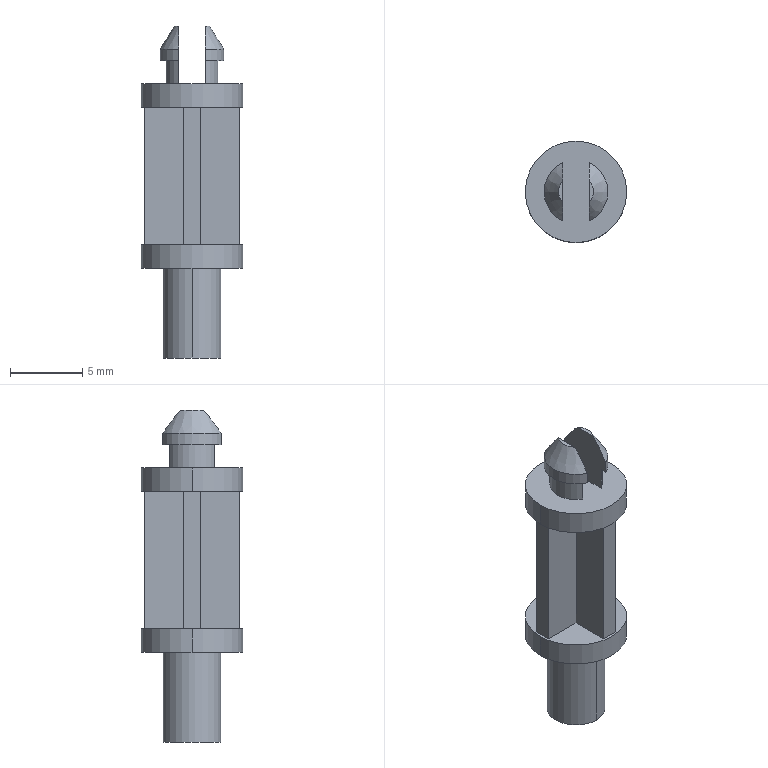Part | STEP file | MSCBSM_M4_8_01 | 1 solid | 35 faces | box 7 x 7 x 22.9 mm | volume 355.891 mm3 | plane 23 | cylinder 10 | cone 2 | commonest cylinder face diameters 7 x4 3.6 x2 4 x2 4.4 x2